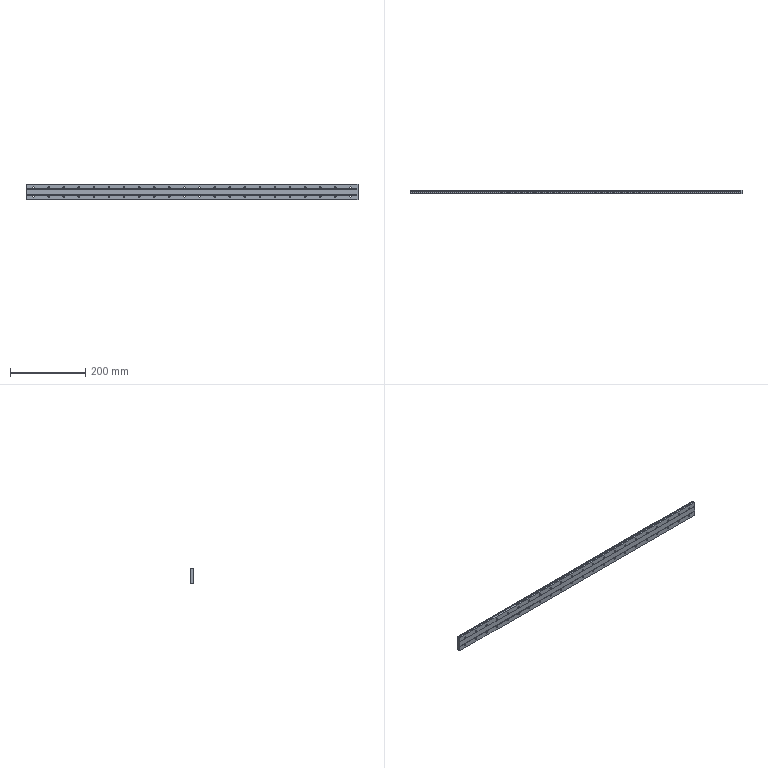Part | STEP file | Linear rail MR15WLSS1V1H-880L-20-20-I(R)_CPC_default | 1 solid | 237 faces | box 880 x 9.5 x 42 mm | volume 319876 mm3 | cylinder 179 | plane 58 | commonest cylinder face diameters 4.5 x88 8 x88 3.18 x3